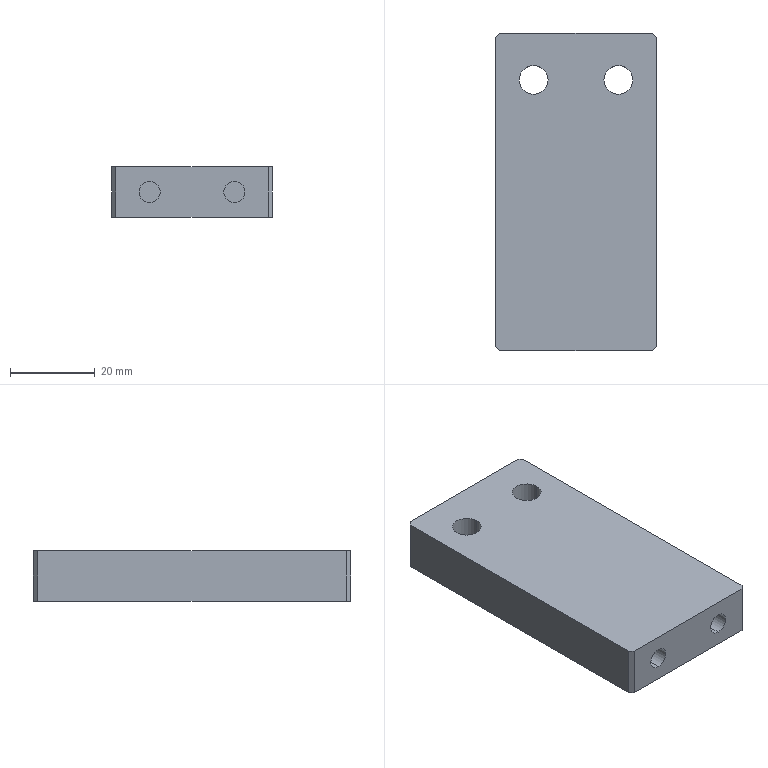Part | SolidWorks | features HoleWzd 3, Chamfer 1, Extrusion 1 | 1 solid | 20 faces | box 38 x 75 x 12 mm | volume 32833 mm3 | plane 12 | cylinder 8 | commonest cylinder face diameters 5 x4 6.8 x4
STEP:
#1=CARTESIAN_POINT('',(-10.,-25.5,2.5));
#2=VERTEX_POINT('',#1);
#3=CARTESIAN_POINT('',(-10.,-25.5,-2.5));
#4=VERTEX_POINT('',#3);
#5=CARTESIAN_POINT('',(-10.,-25.5,0.));
#6=DIRECTION('',(0.,-1.,0.));
#7=DIRECTION('',(0.,0.,-1.));
#8=AXIS2_PLACEMENT_3D('',#5,#6,#7);
#9=CIRCLE('',#8,2.5);
#10=EDGE_CURVE('',#2,#4,#9,.T.);
#11=ORIENTED_EDGE('',*,*,#10,.F.);
#12=CARTESIAN_POINT('',(-10.,-37.5,2.5));
#13=VERTEX_POINT('',#12);
#14=CARTESIAN_POINT('',(-10.,-37.5,2.5));
#15=DIRECTION('',(0.,-1.,0.));
#16=VECTOR('',#15,1000.);
#17=LINE('',#14,#16);
#18=EDGE_CURVE('',#2,#13,#17,.T.);
#19=ORIENTED_EDGE('',*,*,#18,.T.);
#20=CARTESIAN_POINT('',(-10.,-37.5,-2.5));
#21=VERTEX_POINT('',#20);
#22=CARTESIAN_POINT('',(-10.,-37.5,0.));
#23=DIRECTION('',(0.,-1.,0.));
#24=DIRECTION('',(0.,0.,-1.));
#25=AXIS2_PLACEMENT_3D('',#22,#23,#24);
#26=CIRCLE('',#25,2.5);
#27=EDGE_CURVE('',#13,#21,#26,.T.);
#28=ORIENTED_EDGE('',*,*,#27,.T.);
#29=CARTESIAN_POINT('',(-10.,-37.5,-2.5));
#30=DIRECTION('',(0.,-1.,0.));
#31=VECTOR('',#30,1000.);
#32=LINE('',#29,#31);
#33=EDGE_CURVE('',#4,#21,#32,.T.);
#34=ORIENTED_EDGE('',*,*,#33,.F.);
#35=EDGE_LOOP('',(#11,#19,#28,#34));
#36=FACE_OUTER_BOUND('',#35,.T.);
#37=CARTESIAN_POINT('',(-10.,-37.5,0.));
#38=DIRECTION('',(0.,-1.,0.));
#39=DIRECTION('',(0.,0.,-1.));
#40=AXIS2_PLACEMENT_3D('',#37,#38,#39);
#41=CYLINDRICAL_SURFACE('',#40,2.5);
#42=ADVANCED_FACE('',(#36),#41,.F.);
#43=CARTESIAN_POINT('',(10.,-25.5,2.5));
#44=VERTEX_POINT('',#43);
#45=CARTESIAN_POINT('',(10.,-25.5,-2.5));
#46=VERTEX_POINT('',#45);
#47=CARTESIAN_POINT('',(10.,-25.5,0.));
#48=DIRECTION('',(0.,-1.,0.));
#49=DIRECTION('',(0.,0.,-1.));
#50=AXIS2_PLACEMENT_3D('',#47,#48,#49);
#51=CIRCLE('',#50,2.5);
#52=EDGE_CURVE('',#44,#46,#51,.T.);
#53=ORIENTED_EDGE('',*,*,#52,.F.);
#54=CARTESIAN_POINT('',(10.,-37.5,2.5));
#55=VERTEX_POINT('',#54);
#56=CARTESIAN_POINT('',(10.,-37.5,2.5));
#57=DIRECTION('',(0.,-1.,0.));
#58=VECTOR('',#57,1000.);
#59=LINE('',#56,#58);
#60=EDGE_CURVE('',#44,#55,#59,.T.);
#61=ORIENTED_EDGE('',*,*,#60,.T.);
#62=CARTESIAN_POINT('',(10.,-37.5,-2.5));
#63=VERTEX_POINT('',#62);
#64=CARTESIAN_POINT('',(10.,-37.5,0.));
#65=DIRECTION('',(0.,-1.,0.));
#66=DIRECTION('',(0.,0.,-1.));
#67=AXIS2_PLACEMENT_3D('',#64,#65,#66);
#68=CIRCLE('',#67,2.5);
#69=EDGE_CURVE('',#55,#63,#68,.T.);
#70=ORIENTED_EDGE('',*,*,#69,.T.);
#71=CARTESIAN_POINT('',(10.,-37.5,-2.5));
#72=DIRECTION('',(0.,-1.,0.));
#73=VECTOR('',#72,1000.);
#74=LINE('',#71,#73);
#75=EDGE_CURVE('',#46,#63,#74,.T.);
#76=ORIENTED_EDGE('',*,*,#75,.F.);
#77=EDGE_LOOP('',(#53,#61,#70,#76));
#78=FACE_OUTER_BOUND('',#77,.T.);
#79=CARTESIAN_POINT('',(10.,-37.5,0.));
#80=DIRECTION('',(0.,-1.,0.));
#81=DIRECTION('',(0.,0.,-1.));
#82=AXIS2_PLACEMENT_3D('',#79,#80,#81);
#83=CYLINDRICAL_SURFACE('',#82,2.5);
#84=ADVANCED_FACE('',(#78),#83,.F.);
#85=CARTESIAN_POINT('',(6.6,26.5,-6.));
#86=VERTEX_POINT('',#85);
#87=CARTESIAN_POINT('',(13.4,26.5,-6.));
#88=VERTEX_POINT('',#87);
#89=CARTESIAN_POINT('',(10.,26.5,-6.));
#90=DIRECTION('',(0.,0.,1.));
#91=DIRECTION('',(1.,0.,0.));
#92=AXIS2_PLACEMENT_3D('',#89,#90,#91);
#93=CIRCLE('',#92,3.4);
#94=EDGE_CURVE('',#86,#88,#93,.T.);
#95=ORIENTED_EDGE('',*,*,#94,.F.);
#96=CARTESIAN_POINT('',(6.6,26.5,6.));
#97=VERTEX_POINT('',#96);
#98=CARTESIAN_POINT('',(6.6,26.5,6.));
#99=DIRECTION('',(0.,0.,1.));
#100=VECTOR('',#99,1000.);
#101=LINE('',#98,#100);
#102=EDGE_CURVE('',#86,#97,#101,.T.);
#103=ORIENTED_EDGE('',*,*,#102,.T.);
#104=CARTESIAN_POINT('',(13.4,26.5,6.));
#105=VERTEX_POINT('',#104);
#106=CARTESIAN_POINT('',(10.,26.5,6.));
#107=DIRECTION('',(0.,0.,1.));
#108=DIRECTION('',(1.,0.,0.));
#109=AXIS2_PLACEMENT_3D('',#106,#107,#108);
#110=CIRCLE('',#109,3.4);
#111=EDGE_CURVE('',#97,#105,#110,.T.);
#112=ORIENTED_EDGE('',*,*,#111,.T.);
#113=CARTESIAN_POINT('',(13.4,26.5,6.));
#114=DIRECTION('',(0.,0.,1.));
#115=VECTOR('',#114,1000.);
#116=LINE('',#113,#115);
#117=EDGE_CURVE('',#88,#105,#116,.T.);
#118=ORIENTED_EDGE('',*,*,#117,.F.);
#119=EDGE_LOOP('',(#95,#103,#112,#118));
#120=FACE_OUTER_BOUND('',#119,.T.);
#121=CARTESIAN_POINT('',(10.,26.5,6.));
#122=DIRECTION('',(0.,0.,1.));
#123=DIRECTION('',(1.,0.,0.));
#124=AXIS2_PLACEMENT_3D('',#121,#122,#123);
#125=CYLINDRICAL_SURFACE('',#124,3.4);
#126=ADVANCED_FACE('',(#120),#125,.F.);
#127=CARTESIAN_POINT('',(-13.4,26.5,-6.));
#128=VERTEX_POINT('',#127);
#129=CARTESIAN_POINT('',(-6.6,26.5,-6.));
#130=VERTEX_POINT('',#129);
#131=CARTESIAN_POINT('',(-10.,26.5,-6.));
#132=DIRECTION('',(0.,0.,1.));
#133=DIRECTION('',(1.,0.,0.));
#134=AXIS2_PLACEMENT_3D('',#131,#132,#133);
#135=CIRCLE('',#134,3.4);
#136=EDGE_CURVE('',#128,#130,#135,.T.);
#137=ORIENTED_EDGE('',*,*,#136,.F.);
#138=CARTESIAN_POINT('',(-13.4,26.5,6.));
#139=VERTEX_POINT('',#138);
#140=CARTESIAN_POINT('',(-13.4,26.5,6.));
#141=DIRECTION('',(0.,0.,1.));
#142=VECTOR('',#141,1000.);
#143=LINE('',#140,#142);
#144=EDGE_CURVE('',#128,#139,#143,.T.);
#145=ORIENTED_EDGE('',*,*,#144,.T.);
#146=CARTESIAN_POINT('',(-6.6,26.5,6.));
#147=VERTEX_POINT('',#146);
#148=CARTESIAN_POINT('',(-10.,26.5,6.));
#149=DIRECTION('',(0.,0.,1.));
#150=DIRECTION('',(1.,0.,0.));
#151=AXIS2_PLACEMENT_3D('',#148,#149,#150);
#152=CIRCLE('',#151,3.4);
#153=EDGE_CURVE('',#139,#147,#152,.T.);
#154=ORIENTED_EDGE('',*,*,#153,.T.);
#155=CARTESIAN_POINT('',(-6.6,26.5,6.));
#156=DIRECTION('',(0.,0.,1.));
#157=VECTOR('',#156,1000.);
#158=LINE('',#155,#157);
#159=EDGE_CURVE('',#130,#147,#158,.T.);
#160=ORIENTED_EDGE('',*,*,#159,.F.);
#161=EDGE_LOOP('',(#137,#145,#154,#160));
#162=FACE_OUTER_BOUND('',#161,.T.);
#163=CARTESIAN_POINT('',(-10.,26.5,6.));
#164=DIRECTION('',(0.,0.,1.));
#165=DIRECTION('',(1.,0.,0.));
#166=AXIS2_PLACEMENT_3D('',#163,#164,#165);
#167=CYLINDRICAL_SURFACE('',#166,3.4);
#168=ADVANCED_FACE('',(#162),#167,.F.);
#169=CARTESIAN_POINT('',(19.,-36.5,-6.));
#170=VERTEX_POINT('',#169);
#171=CARTESIAN_POINT('',(19.,36.5,-6.));
#172=VERTEX_POINT('',#171);
#173=CARTESIAN_POINT('',(19.,37.5,-6.));
#174=DIRECTION('',(0.,1.,0.));
#175=VECTOR('',#174,1000.);
#176=LINE('',#173,#175);
#177=EDGE_CURVE('',#170,#172,#176,.T.);
#178=ORIENTED_EDGE('',*,*,#177,.T.);
#179=CARTESIAN_POINT('',(19.,36.5,6.));
#180=VERTEX_POINT('',#179);
#181=CARTESIAN_POINT('',(19.,36.5,6.));
#182=DIRECTION('',(0.,0.,1.));
#183=VECTOR('',#182,1000.);
#184=LINE('',#181,#183);
#185=EDGE_CURVE('',#172,#180,#184,.T.);
#186=ORIENTED_EDGE('',*,*,#185,.T.);
#187=CARTESIAN_POINT('',(19.,-36.5,6.));
#188=VERTEX_POINT('',#187);
#189=CARTESIAN_POINT('',(19.,37.5,6.));
#190=DIRECTION('',(0.,1.,0.));
#191=VECTOR('',#190,1000.);
#192=LINE('',#189,#191);
#193=EDGE_CURVE('',#188,#180,#192,.T.);
#194=ORIENTED_EDGE('',*,*,#193,.F.);
#195=CARTESIAN_POINT('',(19.,-36.5,6.));
#196=DIRECTION('',(0.,0.,-1.));
#197=VECTOR('',#196,1000.);
#198=LINE('',#195,#197);
#199=EDGE_CURVE('',#188,#170,#198,.T.);
#200=ORIENTED_EDGE('',*,*,#199,.T.);
#201=EDGE_LOOP('',(#178,#186,#194,#200));
#202=FACE_OUTER_BOUND('',#201,.T.);
#203=CARTESIAN_POINT('',(19.,37.5,6.));
#204=DIRECTION('',(-1.,0.,0.));
#205=DIRECTION('',(0.,-1.,0.));
#206=AXIS2_PLACEMENT_3D('',#203,#204,#205);
#207=PLANE('',#206);
#208=ADVANCED_FACE('',(#202),#207,.F.);
#209=CARTESIAN_POINT('',(18.,37.5,6.));
#210=VERTEX_POINT('',#209);
#211=CARTESIAN_POINT('',(-18.,37.5,6.));
#212=VERTEX_POINT('',#211);
#213=CARTESIAN_POINT('',(-19.,37.5,6.));
#214=DIRECTION('',(-1.,0.,0.));
#215=VECTOR('',#214,1000.);
#216=LINE('',#213,#215);
#217=EDGE_CURVE('',#210,#212,#216,.T.);
#218=ORIENTED_EDGE('',*,*,#217,.F.);
#219=CARTESIAN_POINT('',(18.,37.5,-6.));
#220=VERTEX_POINT('',#219);
#221=CARTESIAN_POINT('',(18.,37.5,6.));
#222=DIRECTION('',(0.,0.,-1.));
#223=VECTOR('',#222,1000.);
#224=LINE('',#221,#223);
#225=EDGE_CURVE('',#210,#220,#224,.T.);
#226=ORIENTED_EDGE('',*,*,#225,.T.);
#227=CARTESIAN_POINT('',(-18.,37.5,-6.));
#228=VERTEX_POINT('',#227);
#229=CARTESIAN_POINT('',(-19.,37.5,-6.));
#230=DIRECTION('',(-1.,0.,0.));
#231=VECTOR('',#230,1000.);
#232=LINE('',#229,#231);
#233=EDGE_CURVE('',#220,#228,#232,.T.);
#234=ORIENTED_EDGE('',*,*,#233,.T.);
#235=CARTESIAN_POINT('',(-18.,37.5,6.));
#236=DIRECTION('',(0.,0.,1.));
#237=VECTOR('',#236,1000.);
#238=LINE('',#235,#237);
#239=EDGE_CURVE('',#228,#212,#238,.T.);
#240=ORIENTED_EDGE('',*,*,#239,.T.);
#241=EDGE_LOOP('',(#218,#226,#234,#240));
#242=FACE_OUTER_BOUND('',#241,.T.);
#243=CARTESIAN_POINT('',(-19.,37.5,6.));
#244=DIRECTION('',(0.,-1.,0.));
#245=DIRECTION('',(0.,0.,-1.));
#246=AXIS2_PLACEMENT_3D('',#243,#244,#245);
#247=PLANE('',#246);
#248=ADVANCED_FACE('',(#242),#247,.F.);
#249=CARTESIAN_POINT('',(-19.,36.5,6.));
#250=VERTEX_POINT('',#249);
#251=CARTESIAN_POINT('',(-19.,-36.5,6.));
#252=VERTEX_POINT('',#251);
#253=CARTESIAN_POINT('',(-19.,37.5,6.));
#254=DIRECTION('',(0.,-1.,0.));
#255=VECTOR('',#254,1000.);
#256=LINE('',#253,#255);
#257=EDGE_CURVE('',#250,#252,#256,.T.);
#258=ORIENTED_EDGE('',*,*,#257,.F.);
#259=CARTESIAN_POINT('',(-19.,36.5,-6.));
#260=VERTEX_POINT('',#259);
#261=CARTESIAN_POINT('',(-19.,36.5,6.));
#262=DIRECTION('',(0.,0.,-1.));
#263=VECTOR('',#262,1000.);
#264=LINE('',#261,#263);
#265=EDGE_CURVE('',#250,#260,#264,.T.);
#266=ORIENTED_EDGE('',*,*,#265,.T.);
#267=CARTESIAN_POINT('',(-19.,-36.5,-6.));
#268=VERTEX_POINT('',#267);
#269=CARTESIAN_POINT('',(-19.,37.5,-6.));
#270=DIRECTION('',(0.,-1.,0.));
#271=VECTOR('',#270,1000.);
#272=LINE('',#269,#271);
#273=EDGE_CURVE('',#260,#268,#272,.T.);
#274=ORIENTED_EDGE('',*,*,#273,.T.);
#275=CARTESIAN_POINT('',(-19.,-36.5,6.));
#276=DIRECTION('',(0.,0.,1.));
#277=VECTOR('',#276,1000.);
#278=LINE('',#275,#277);
#279=EDGE_CURVE('',#268,#252,#278,.T.);
#280=ORIENTED_EDGE('',*,*,#279,.T.);
#281=EDGE_LOOP('',(#258,#266,#274,#280));
#282=FACE_OUTER_BOUND('',#281,.T.);
#283=CARTESIAN_POINT('',(-19.,37.5,6.));
#284=DIRECTION('',(1.,0.,0.));
#285=DIRECTION('',(0.,1.,0.));
#286=AXIS2_PLACEMENT_3D('',#283,#284,#285);
#287=PLANE('',#286);
#288=ADVANCED_FACE('',(#282),#287,.F.);
#289=CARTESIAN_POINT('',(-10.,-37.5,0.));
#290=DIRECTION('',(0.,-1.,0.));
#291=DIRECTION('',(0.,0.,-1.));
#292=AXIS2_PLACEMENT_3D('',#289,#290,#291);
#293=CIRCLE('',#292,2.5);
#294=EDGE_CURVE('',#21,#13,#293,.T.);
#295=ORIENTED_EDGE('',*,*,#294,.F.);
#296=ORIENTED_EDGE('',*,*,#27,.F.);
#297=EDGE_LOOP('',(#295,#296));
#298=FACE_BOUND('',#297,.T.);
#299=CARTESIAN_POINT('',(10.,-37.5,0.));
#300=DIRECTION('',(0.,-1.,0.));
#301=DIRECTION('',(0.,0.,-1.));
#302=AXIS2_PLACEMENT_3D('',#299,#300,#301);
#303=CIRCLE('',#302,2.5);
#304=EDGE_CURVE('',#63,#55,#303,.T.);
#305=ORIENTED_EDGE('',*,*,#304,.F.);
#306=ORIENTED_EDGE('',*,*,#69,.F.);
#307=EDGE_LOOP('',(#305,#306));
#308=FACE_BOUND('',#307,.T.);
#309=CARTESIAN_POINT('',(-18.,-37.5,6.));
#310=VERTEX_POINT('',#309);
#311=CARTESIAN_POINT('',(18.,-37.5,6.));
#312=VERTEX_POINT('',#311);
#313=CARTESIAN_POINT('',(-19.,-37.5,6.));
#314=DIRECTION('',(1.,0.,0.));
#315=VECTOR('',#314,1000.);
#316=LINE('',#313,#315);
#317=EDGE_CURVE('',#310,#312,#316,.T.);
#318=ORIENTED_EDGE('',*,*,#317,.F.);
#319=CARTESIAN_POINT('',(-18.,-37.5,-6.));
#320=VERTEX_POINT('',#319);
#321=CARTESIAN_POINT('',(-18.,-37.5,6.));
#322=DIRECTION('',(0.,0.,-1.));
#323=VECTOR('',#322,1000.);
#324=LINE('',#321,#323);
#325=EDGE_CURVE('',#310,#320,#324,.T.);
#326=ORIENTED_EDGE('',*,*,#325,.T.);
#327=CARTESIAN_POINT('',(18.,-37.5,-6.));
#328=VERTEX_POINT('',#327);
#329=CARTESIAN_POINT('',(-19.,-37.5,-6.));
#330=DIRECTION('',(1.,0.,0.));
#331=VECTOR('',#330,1000.);
#332=LINE('',#329,#331);
#333=EDGE_CURVE('',#320,#328,#332,.T.);
#334=ORIENTED_EDGE('',*,*,#333,.T.);
#335=CARTESIAN_POINT('',(18.,-37.5,6.));
#336=DIRECTION('',(0.,0.,1.));
#337=VECTOR('',#336,1000.);
#338=LINE('',#335,#337);
#339=EDGE_CURVE('',#328,#312,#338,.T.);
#340=ORIENTED_EDGE('',*,*,#339,.T.);
#341=EDGE_LOOP('',(#318,#326,#334,#340));
#342=FACE_OUTER_BOUND('',#341,.T.);
#343=CARTESIAN_POINT('',(-19.,-37.5,6.));
#344=DIRECTION('',(0.,1.,0.));
#345=DIRECTION('',(0.,0.,1.));
#346=AXIS2_PLACEMENT_3D('',#343,#344,#345);
#347=PLANE('',#346);
#348=ADVANCED_FACE('',(#298,#308,#342),#347,.F.);
#349=CARTESIAN_POINT('',(10.,26.5,6.));
#350=DIRECTION('',(0.,0.,1.));
#351=DIRECTION('',(1.,0.,0.));
#352=AXIS2_PLACEMENT_3D('',#349,#350,#351);
#353=CIRCLE('',#352,3.4);
#354=EDGE_CURVE('',#105,#97,#353,.T.);
#355=ORIENTED_EDGE('',*,*,#354,.F.);
#356=ORIENTED_EDGE('',*,*,#111,.F.);
#357=EDGE_LOOP('',(#355,#356));
#358=FACE_BOUND('',#357,.T.);
#359=CARTESIAN_POINT('',(-10.,26.5,6.));
#360=DIRECTION('',(0.,0.,1.));
#361=DIRECTION('',(1.,0.,0.));
#362=AXIS2_PLACEMENT_3D('',#359,#360,#361);
#363=CIRCLE('',#362,3.4);
#364=EDGE_CURVE('',#147,#139,#363,.T.);
#365=ORIENTED_EDGE('',*,*,#364,.F.);
#366=ORIENTED_EDGE('',*,*,#153,.F.);
#367=EDGE_LOOP('',(#365,#366));
#368=FACE_BOUND('',#367,.T.);
#369=ORIENTED_EDGE('',*,*,#193,.T.);
#370=CARTESIAN_POINT('',(27.75,27.75,6.));
#371=DIRECTION('',(-0.7071,0.7071,0.));
#372=VECTOR('',#371,1000.);
#373=LINE('',#370,#372);
#374=EDGE_CURVE('',#180,#210,#373,.T.);
#375=ORIENTED_EDGE('',*,*,#374,.T.);
#376=ORIENTED_EDGE('',*,*,#217,.T.);
#377=CARTESIAN_POINT('',(-27.75,27.75,6.));
#378=DIRECTION('',(-0.7071,-0.7071,0.));
#379=VECTOR('',#378,1000.);
#380=LINE('',#377,#379);
#381=EDGE_CURVE('',#212,#250,#380,.T.);
#382=ORIENTED_EDGE('',*,*,#381,.T.);
#383=ORIENTED_EDGE('',*,*,#257,.T.);
#384=CARTESIAN_POINT('',(-27.75,-27.75,6.));
#385=DIRECTION('',(0.7071,-0.7071,0.));
#386=VECTOR('',#385,1000.);
#387=LINE('',#384,#386);
#388=EDGE_CURVE('',#252,#310,#387,.T.);
#389=ORIENTED_EDGE('',*,*,#388,.T.);
#390=ORIENTED_EDGE('',*,*,#317,.T.);
#391=CARTESIAN_POINT('',(27.75,-27.75,6.));
#392=DIRECTION('',(0.7071,0.7071,0.));
#393=VECTOR('',#392,1000.);
#394=LINE('',#391,#393);
#395=EDGE_CURVE('',#312,#188,#394,.T.);
#396=ORIENTED_EDGE('',*,*,#395,.T.);
#397=EDGE_LOOP('',(#369,#375,#376,#382,#383,#389,#390,#396));
#398=FACE_OUTER_BOUND('',#397,.T.);
#399=CARTESIAN_POINT('',(0.,0.,6.));
#400=DIRECTION('',(0.,0.,1.));
#401=DIRECTION('',(1.,0.,0.));
#402=AXIS2_PLACEMENT_3D('',#399,#400,#401);
#403=PLANE('',#402);
#404=ADVANCED_FACE('',(#358,#368,#398),#403,.T.);
#405=CARTESIAN_POINT('',(10.,26.5,-6.));
#406=DIRECTION('',(0.,0.,1.));
#407=DIRECTION('',(1.,0.,0.));
#408=AXIS2_PLACEMENT_3D('',#405,#406,#407);
#409=CIRCLE('',#408,3.4);
#410=EDGE_CURVE('',#88,#86,#409,.T.);
#411=ORIENTED_EDGE('',*,*,#410,.T.);
#412=ORIENTED_EDGE('',*,*,#94,.T.);
#413=EDGE_LOOP('',(#411,#412));
#414=FACE_BOUND('',#413,.T.);
#415=CARTESIAN_POINT('',(-10.,26.5,-6.));
#416=DIRECTION('',(0.,0.,1.));
#417=DIRECTION('',(1.,0.,0.));
#418=AXIS2_PLACEMENT_3D('',#415,#416,#417);
#419=CIRCLE('',#418,3.4);
#420=EDGE_CURVE('',#130,#128,#419,.T.);
#421=ORIENTED_EDGE('',*,*,#420,.T.);
#422=ORIENTED_EDGE('',*,*,#136,.T.);
#423=EDGE_LOOP('',(#421,#422));
#424=FACE_BOUND('',#423,.T.);
#425=ORIENTED_EDGE('',*,*,#233,.F.);
#426=CARTESIAN_POINT('',(18.,37.5,-6.));
#427=DIRECTION('',(0.7071,-0.7071,0.));
#428=VECTOR('',#427,1000.);
#429=LINE('',#426,#428);
#430=EDGE_CURVE('',#220,#172,#429,.T.);
#431=ORIENTED_EDGE('',*,*,#430,.T.);
#432=ORIENTED_EDGE('',*,*,#177,.F.);
#433=CARTESIAN_POINT('',(19.,-36.5,-6.));
#434=DIRECTION('',(-0.7071,-0.7071,0.));
#435=VECTOR('',#434,1000.);
#436=LINE('',#433,#435);
#437=EDGE_CURVE('',#170,#328,#436,.T.);
#438=ORIENTED_EDGE('',*,*,#437,.T.);
#439=ORIENTED_EDGE('',*,*,#333,.F.);
#440=CARTESIAN_POINT('',(-18.,-37.5,-6.));
#441=DIRECTION('',(-0.7071,0.7071,0.));
#442=VECTOR('',#441,1000.);
#443=LINE('',#440,#442);
#444=EDGE_CURVE('',#320,#268,#443,.T.);
#445=ORIENTED_EDGE('',*,*,#444,.T.);
#446=ORIENTED_EDGE('',*,*,#273,.F.);
#447=CARTESIAN_POINT('',(-19.,36.5,-6.));
#448=DIRECTION('',(0.7071,0.7071,0.));
#449=VECTOR('',#448,1000.);
#450=LINE('',#447,#449);
#451=EDGE_CURVE('',#260,#228,#450,.T.);
#452=ORIENTED_EDGE('',*,*,#451,.T.);
#453=EDGE_LOOP('',(#425,#431,#432,#438,#439,#445,#446,#452));
#454=FACE_OUTER_BOUND('',#453,.T.);
#455=CARTESIAN_POINT('',(0.,0.,-6.));
#456=DIRECTION('',(0.,0.,1.));
#457=DIRECTION('',(1.,0.,0.));
#458=AXIS2_PLACEMENT_3D('',#455,#456,#457);
#459=PLANE('',#458);
#460=ADVANCED_FACE('',(#414,#424,#454),#459,.F.);
#461=ORIENTED_EDGE('',*,*,#144,.F.);
#462=ORIENTED_EDGE('',*,*,#420,.F.);
#463=ORIENTED_EDGE('',*,*,#159,.T.);
#464=ORIENTED_EDGE('',*,*,#364,.T.);
#465=EDGE_LOOP('',(#461,#462,#463,#464));
#466=FACE_OUTER_BOUND('',#465,.T.);
#467=CARTESIAN_POINT('',(-10.,26.5,6.));
#468=DIRECTION('',(0.,0.,1.));
#469=DIRECTION('',(1.,0.,0.));
#470=AXIS2_PLACEMENT_3D('',#467,#468,#469);
#471=CYLINDRICAL_SURFACE('',#470,3.4);
#472=ADVANCED_FACE('',(#466),#471,.F.);
#473=ORIENTED_EDGE('',*,*,#102,.F.);
#474=ORIENTED_EDGE('',*,*,#410,.F.);
#475=ORIENTED_EDGE('',*,*,#117,.T.);
#476=ORIENTED_EDGE('',*,*,#354,.T.);
#477=EDGE_LOOP('',(#473,#474,#475,#476));
#478=FACE_OUTER_BOUND('',#477,.T.);
#479=CARTESIAN_POINT('',(10.,26.5,6.));
#480=DIRECTION('',(0.,0.,1.));
#481=DIRECTION('',(1.,0.,0.));
#482=AXIS2_PLACEMENT_3D('',#479,#480,#481);
#483=CYLINDRICAL_SURFACE('',#482,3.4);
#484=ADVANCED_FACE('',(#478),#483,.F.);
#485=CARTESIAN_POINT('',(10.,-25.5,0.));
#486=DIRECTION('',(0.,-1.,0.));
#487=DIRECTION('',(0.,0.,-1.));
#488=AXIS2_PLACEMENT_3D('',#485,#486,#487);
#489=CIRCLE('',#488,2.5);
#490=EDGE_CURVE('',#46,#44,#489,.T.);
#491=ORIENTED_EDGE('',*,*,#490,.T.);
#492=ORIENTED_EDGE('',*,*,#52,.T.);
#493=EDGE_LOOP('',(#491,#492));
#494=FACE_OUTER_BOUND('',#493,.T.);
#495=CARTESIAN_POINT('',(10.,-25.5,0.));
#496=DIRECTION('',(0.,1.,0.));
#497=DIRECTION('',(0.,0.,1.));
#498=AXIS2_PLACEMENT_3D('',#495,#496,#497);
#499=PLANE('',#498);
#500=ADVANCED_FACE('',(#494),#499,.F.);
#501=ORIENTED_EDGE('',*,*,#60,.F.);
#502=ORIENTED_EDGE('',*,*,#490,.F.);
#503=ORIENTED_EDGE('',*,*,#75,.T.);
#504=ORIENTED_EDGE('',*,*,#304,.T.);
#505=EDGE_LOOP('',(#501,#502,#503,#504));
#506=FACE_OUTER_BOUND('',#505,.T.);
#507=CARTESIAN_POINT('',(10.,-37.5,0.));
#508=DIRECTION('',(0.,-1.,0.));
#509=DIRECTION('',(0.,0.,-1.));
#510=AXIS2_PLACEMENT_3D('',#507,#508,#509);
#511=CYLINDRICAL_SURFACE('',#510,2.5);
#512=ADVANCED_FACE('',(#506),#511,.F.);
#513=CARTESIAN_POINT('',(-10.,-25.5,0.));
#514=DIRECTION('',(0.,-1.,0.));
#515=DIRECTION('',(0.,0.,-1.));
#516=AXIS2_PLACEMENT_3D('',#513,#514,#515);
#517=CIRCLE('',#516,2.5);
#518=EDGE_CURVE('',#4,#2,#517,.T.);
#519=ORIENTED_EDGE('',*,*,#518,.T.);
#520=ORIENTED_EDGE('',*,*,#10,.T.);
#521=EDGE_LOOP('',(#519,#520));
#522=FACE_OUTER_BOUND('',#521,.T.);
#523=CARTESIAN_POINT('',(-10.,-25.5,0.));
#524=DIRECTION('',(0.,1.,0.));
#525=DIRECTION('',(0.,0.,1.));
#526=AXIS2_PLACEMENT_3D('',#523,#524,#525);
#527=PLANE('',#526);
#528=ADVANCED_FACE('',(#522),#527,.F.);
#529=ORIENTED_EDGE('',*,*,#18,.F.);
#530=ORIENTED_EDGE('',*,*,#518,.F.);
#531=ORIENTED_EDGE('',*,*,#33,.T.);
#532=ORIENTED_EDGE('',*,*,#294,.T.);
#533=EDGE_LOOP('',(#529,#530,#531,#532));
#534=FACE_OUTER_BOUND('',#533,.T.);
#535=CARTESIAN_POINT('',(-10.,-37.5,0.));
#536=DIRECTION('',(0.,-1.,0.));
#537=DIRECTION('',(0.,0.,-1.));
#538=AXIS2_PLACEMENT_3D('',#535,#536,#537);
#539=CYLINDRICAL_SURFACE('',#538,2.5);
#540=ADVANCED_FACE('',(#534),#539,.F.);
#541=ORIENTED_EDGE('',*,*,#374,.F.);
#542=ORIENTED_EDGE('',*,*,#185,.F.);
#543=ORIENTED_EDGE('',*,*,#430,.F.);
#544=ORIENTED_EDGE('',*,*,#225,.F.);
#545=EDGE_LOOP('',(#541,#542,#543,#544));
#546=FACE_OUTER_BOUND('',#545,.T.);
#547=CARTESIAN_POINT('',(18.,37.5,6.));
#548=DIRECTION('',(-0.7071,-0.7071,0.));
#549=DIRECTION('',(0.,0.,-1.));
#550=AXIS2_PLACEMENT_3D('',#547,#548,#549);
#551=PLANE('',#550);
#552=ADVANCED_FACE('',(#546),#551,.F.);
#553=ORIENTED_EDGE('',*,*,#381,.F.);
#554=ORIENTED_EDGE('',*,*,#239,.F.);
#555=ORIENTED_EDGE('',*,*,#451,.F.);
#556=ORIENTED_EDGE('',*,*,#265,.F.);
#557=EDGE_LOOP('',(#553,#554,#555,#556));
#558=FACE_OUTER_BOUND('',#557,.T.);
#559=CARTESIAN_POINT('',(-19.,36.5,6.));
#560=DIRECTION('',(0.7071,-0.7071,0.));
#561=DIRECTION('',(0.,0.,-1.));
#562=AXIS2_PLACEMENT_3D('',#559,#560,#561);
#563=PLANE('',#562);
#564=ADVANCED_FACE('',(#558),#563,.F.);
#565=ORIENTED_EDGE('',*,*,#388,.F.);
#566=ORIENTED_EDGE('',*,*,#279,.F.);
#567=ORIENTED_EDGE('',*,*,#444,.F.);
#568=ORIENTED_EDGE('',*,*,#325,.F.);
#569=EDGE_LOOP('',(#565,#566,#567,#568));
#570=FACE_OUTER_BOUND('',#569,.T.);
#571=CARTESIAN_POINT('',(-18.,-37.5,6.));
#572=DIRECTION('',(0.7071,0.7071,0.));
#573=DIRECTION('',(0.,0.,-1.));
#574=AXIS2_PLACEMENT_3D('',#571,#572,#573);
#575=PLANE('',#574);
#576=ADVANCED_FACE('',(#570),#575,.F.);
#577=ORIENTED_EDGE('',*,*,#395,.F.);
#578=ORIENTED_EDGE('',*,*,#339,.F.);
#579=ORIENTED_EDGE('',*,*,#437,.F.);
#580=ORIENTED_EDGE('',*,*,#199,.F.);
#581=EDGE_LOOP('',(#577,#578,#579,#580));
#582=FACE_OUTER_BOUND('',#581,.T.);
#583=CARTESIAN_POINT('',(19.,-36.5,6.));
#584=DIRECTION('',(-0.7071,0.7071,0.));
#585=DIRECTION('',(0.,0.,-1.));
#586=AXIS2_PLACEMENT_3D('',#583,#584,#585);
#587=PLANE('',#586);
#588=ADVANCED_FACE('',(#582),#587,.F.);
#589=CLOSED_SHELL('',(#42,#84,#126,#168,#208,#248,#288,#348,#404,#460,#472,#484,#500,#512,#528,#540,#552,#564,#576,#588));
#590=MANIFOLD_SOLID_BREP('',#589);
#591=CARTESIAN_POINT('',(0.,0.,0.));
#592=DIRECTION('',(0.,0.,1.));
#593=DIRECTION('',(1.,0.,0.));
#594=AXIS2_PLACEMENT_3D('',#591,#592,#593);
#595=(LENGTH_UNIT()NAMED_UNIT(*)SI_UNIT(.MILLI.,.METRE.));
#596=UNCERTAINTY_MEASURE_WITH_UNIT(LENGTH_MEASURE(0.00001),#595,'','');
#597=(NAMED_UNIT(*)PLANE_ANGLE_UNIT()SI_UNIT($,.RADIAN.));
#598=(NAMED_UNIT(*)SI_UNIT($,.STERADIAN.)SOLID_ANGLE_UNIT());
#599=(GEOMETRIC_REPRESENTATION_CONTEXT(3)GLOBAL_UNCERTAINTY_ASSIGNED_CONTEXT((#596))GLOBAL_UNIT_ASSIGNED_CONTEXT((#595,#597,#598))REPRESENTATION_CONTEXT('',''));
#600=ADVANCED_BREP_SHAPE_REPRESENTATION('',(#590,#594),#599);